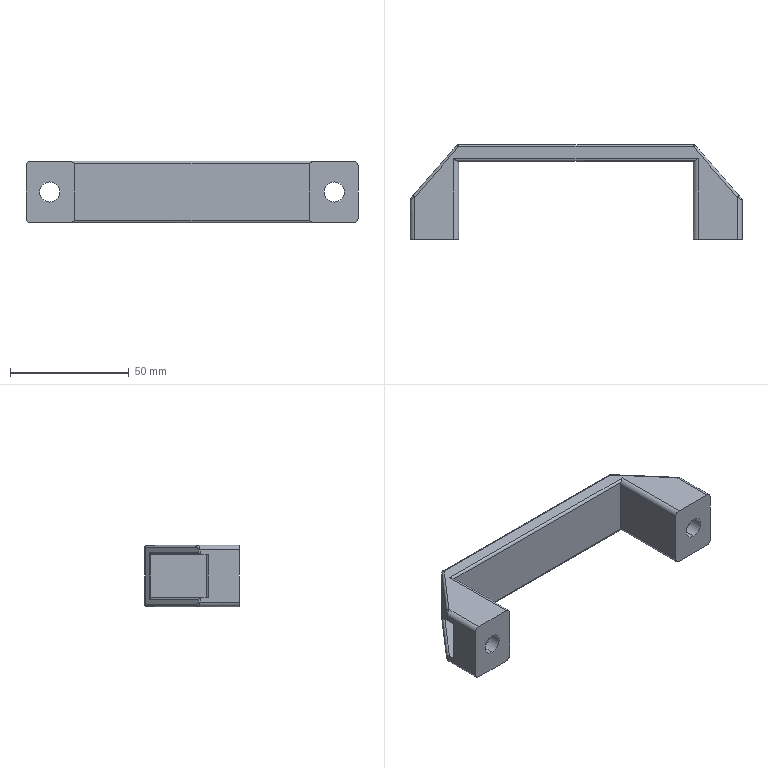Part | SolidWorks | features ICE 3, Fillet 2, Extrusion 1, HoleWzd 1, MirrorPattern 1 | 1 solid | 68 faces | box 140 x 40 x 26 mm | volume 36488 mm3 | cylinder 38 | plane 22 | spline 4 | sphere 4 | commonest cylinder face diameters 2 x22 4 x8 8.5 x4 14 x4